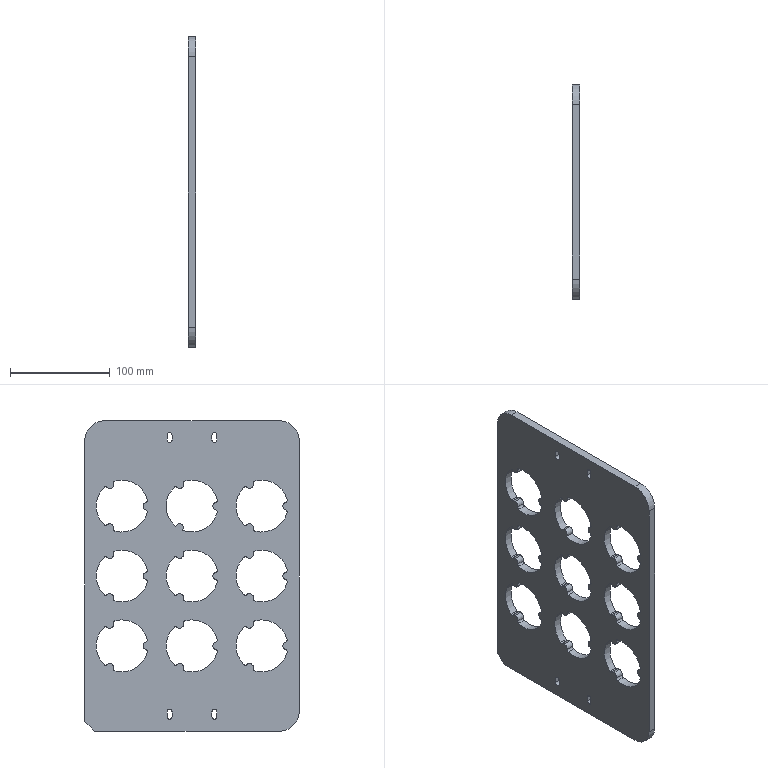Part | SolidWorks | features Cut 2, Fillet 2, ICE 2, MirrorPattern 2, MoveFace 2, Chamfer 1, Extrusion 1, LPattern 1 | 1 solid | 173 faces | box 8 x 215 x 311 mm | volume 385506 mm3 | cylinder 156 | plane 17 | commonest cylinder face diameters 4 x69 8 x36 52 x36 5 x12 40 x3